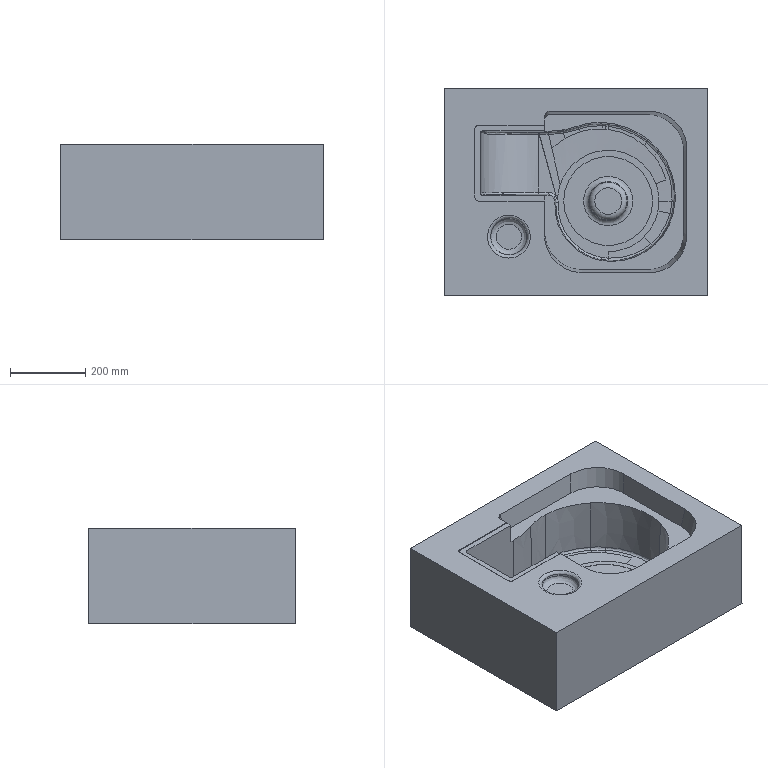Part | 1 solid | 91 faces | box 700 x 550 x 255 mm | volume 69601555 mm3 | plane 26 | spline 23 | cylinder 19 | cone 12 | torus 11 | commonest cylinder face diameters 12.72 x6 12.721 x3 200 x3 12.716 x1 12.719 x1 12.724 x1